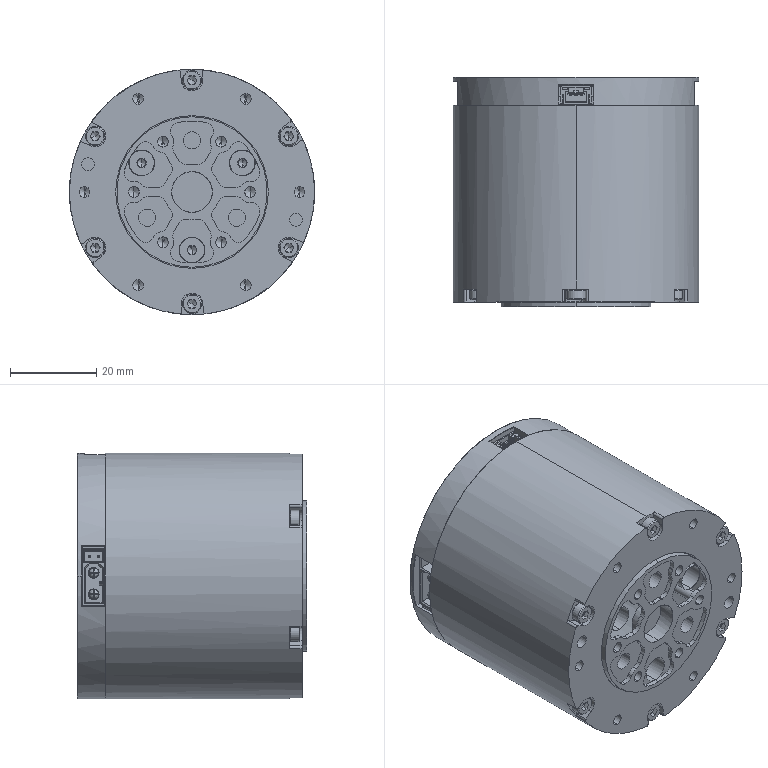Part | SolidWorks | 2 solids | 2128 faces | box 57 x 53.3 x 57 mm | volume 118253 mm3 | plane 1126 | cylinder 704 | cone 179 | spline 105 | torus 14 | commonest cylinder face diameters 4 x106 0.254 x96 2.5 x74 2.28 x72 2.05 x38 5 x24